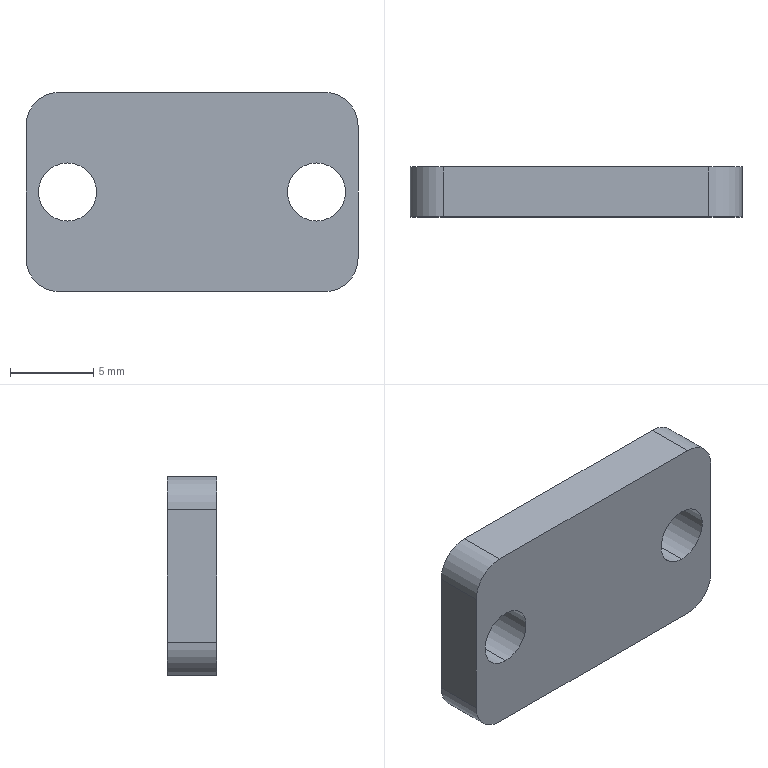Part | STEP file | MGN9C short slider pad plate 1001 | 1 solid | 14 faces | box 20 x 3 x 12 mm | volume 651.972 mm3 | cylinder 8 | plane 6 | commonest cylinder face diameters 3.5 x4 4 x4
STEP:
#1=CARTESIAN_POINT('',(0.,0.,0.));
#2=DIRECTION('',(0.,0.,1.));
#3=DIRECTION('',(1.,0.,0.));
#4=AXIS2_PLACEMENT_3D('',#1,#2,#3);
#5=CARTESIAN_POINT('',(7.5,3.,-1.75));
#6=VERTEX_POINT('',#5);
#7=CARTESIAN_POINT('',(7.5,0.,-1.75));
#8=VERTEX_POINT('',#7);
#9=CARTESIAN_POINT('',(7.5,3.,-1.75));
#10=DIRECTION('',(0.,-1.,0.));
#11=VECTOR('',#10,1.);
#12=LINE('',#9,#11);
#13=CARTESIAN_POINT('',(7.5,3.,0.));
#14=DIRECTION('',(0.,-1.,0.));
#15=DIRECTION('',(0.,0.,-1.));
#16=AXIS2_PLACEMENT_3D('',#13,#14,#15);
#17=CYLINDRICAL_SURFACE('',#16,1.75);
#18=CARTESIAN_POINT('',(6.283,0.));
#19=DIRECTION('',(0.,1.));
#20=VECTOR('',#19,1.);
#21=LINE('',#18,#20);
#22=(GEOMETRIC_REPRESENTATION_CONTEXT(2)PARAMETRIC_REPRESENTATION_CONTEXT()REPRESENTATION_CONTEXT('',''));
#23=DEFINITIONAL_REPRESENTATION('',(#21),#22);
#24=PCURVE('',#17,#23);
#25=CARTESIAN_POINT('',(7.5,3.,0.));
#26=DIRECTION('',(0.,-1.,0.));
#27=DIRECTION('',(0.,0.,-1.));
#28=AXIS2_PLACEMENT_3D('',#25,#26,#27);
#29=CYLINDRICAL_SURFACE('',#28,1.75);
#30=CARTESIAN_POINT('',(0.,0.));
#31=DIRECTION('',(0.,1.));
#32=VECTOR('',#31,1.);
#33=LINE('',#30,#32);
#34=(GEOMETRIC_REPRESENTATION_CONTEXT(2)PARAMETRIC_REPRESENTATION_CONTEXT()REPRESENTATION_CONTEXT('',''));
#35=DEFINITIONAL_REPRESENTATION('',(#33),#34);
#36=PCURVE('',#29,#35);
#37=SURFACE_CURVE('',#12,(#24,#36),.PCURVE_S1.);
#38=EDGE_CURVE('',#6,#8,#37,.T.);
#39=ORIENTED_EDGE('',*,*,#38,.T.);
#40=CARTESIAN_POINT('',(7.5,0.,1.75));
#41=VERTEX_POINT('',#40);
#42=CARTESIAN_POINT('',(7.5,0.,0.));
#43=DIRECTION('',(0.,1.,0.));
#44=DIRECTION('',(0.,0.,-1.));
#45=AXIS2_PLACEMENT_3D('',#42,#43,#44);
#46=CIRCLE('',#45,1.75);
#47=CARTESIAN_POINT('',(6.283,3.));
#48=DIRECTION('',(-1.,0.));
#49=VECTOR('',#48,1.);
#50=LINE('',#47,#49);
#51=(GEOMETRIC_REPRESENTATION_CONTEXT(2)PARAMETRIC_REPRESENTATION_CONTEXT()REPRESENTATION_CONTEXT('',''));
#52=DEFINITIONAL_REPRESENTATION('',(#50),#51);
#53=PCURVE('',#17,#52);
#54=CARTESIAN_POINT('',(0.,0.,0.));
#55=DIRECTION('',(0.,-1.,0.));
#56=DIRECTION('',(0.,0.,-1.));
#57=AXIS2_PLACEMENT_3D('',#54,#55,#56);
#58=PLANE('',#57);
#59=CARTESIAN_POINT('',(1.75,7.5));
#60=CARTESIAN_POINT('',(1.75,4.469));
#61=CARTESIAN_POINT('',(-0.875,5.984));
#62=CARTESIAN_POINT('',(-3.5,7.5));
#63=CARTESIAN_POINT('',(-0.875,9.016));
#64=CARTESIAN_POINT('',(1.75,10.531));
#65=CARTESIAN_POINT('',(1.75,7.5));
#66=(BOUNDED_CURVE()B_SPLINE_CURVE(2,(#59,#60,#61,#62,#63,#64,#65),.UNSPECIFIED.,.T.,.F.)B_SPLINE_CURVE_WITH_KNOTS((1,2,2,2,2,1),(-2.094,0.,2.094,4.189,6.283,8.378),.UNSPECIFIED.)CURVE()GEOMETRIC_REPRESENTATION_ITEM()RATIONAL_B_SPLINE_CURVE((1.,0.5,1.,0.5,1.,0.5,1.))REPRESENTATION_ITEM(''));
#67=(GEOMETRIC_REPRESENTATION_CONTEXT(2)PARAMETRIC_REPRESENTATION_CONTEXT()REPRESENTATION_CONTEXT('',''));
#68=DEFINITIONAL_REPRESENTATION('',(#66),#67);
#69=PCURVE('',#58,#68);
#70=SURFACE_CURVE('',#46,(#53,#69),.PCURVE_S1.);
#71=EDGE_CURVE('',#8,#41,#70,.T.);
#72=ORIENTED_EDGE('',*,*,#71,.T.);
#73=CARTESIAN_POINT('',(7.5,3.,1.75));
#74=VERTEX_POINT('',#73);
#75=CARTESIAN_POINT('',(7.5,3.,1.75));
#76=DIRECTION('',(0.,-1.,0.));
#77=VECTOR('',#76,1.);
#78=LINE('',#75,#77);
#79=CARTESIAN_POINT('',(3.142,0.));
#80=DIRECTION('',(0.,1.));
#81=VECTOR('',#80,1.);
#82=LINE('',#79,#81);
#83=(GEOMETRIC_REPRESENTATION_CONTEXT(2)PARAMETRIC_REPRESENTATION_CONTEXT()REPRESENTATION_CONTEXT('',''));
#84=DEFINITIONAL_REPRESENTATION('',(#82),#83);
#85=PCURVE('',#17,#84);
#86=CARTESIAN_POINT('',(3.142,0.));
#87=DIRECTION('',(0.,1.));
#88=VECTOR('',#87,1.);
#89=LINE('',#86,#88);
#90=(GEOMETRIC_REPRESENTATION_CONTEXT(2)PARAMETRIC_REPRESENTATION_CONTEXT()REPRESENTATION_CONTEXT('',''));
#91=DEFINITIONAL_REPRESENTATION('',(#89),#90);
#92=PCURVE('',#29,#91);
#93=SURFACE_CURVE('',#78,(#85,#92),.PCURVE_S1.);
#94=EDGE_CURVE('',#74,#41,#93,.T.);
#95=ORIENTED_EDGE('',*,*,#94,.F.);
#96=CARTESIAN_POINT('',(7.5,3.,0.));
#97=DIRECTION('',(0.,1.,0.));
#98=DIRECTION('',(0.,0.,-1.));
#99=AXIS2_PLACEMENT_3D('',#96,#97,#98);
#100=CIRCLE('',#99,1.75);
#101=CARTESIAN_POINT('',(6.283,0.));
#102=DIRECTION('',(-1.,0.));
#103=VECTOR('',#102,1.);
#104=LINE('',#101,#103);
#105=(GEOMETRIC_REPRESENTATION_CONTEXT(2)PARAMETRIC_REPRESENTATION_CONTEXT()REPRESENTATION_CONTEXT('',''));
#106=DEFINITIONAL_REPRESENTATION('',(#104),#105);
#107=PCURVE('',#17,#106);
#108=CARTESIAN_POINT('',(0.,3.,0.));
#109=DIRECTION('',(0.,-1.,0.));
#110=DIRECTION('',(0.,0.,-1.));
#111=AXIS2_PLACEMENT_3D('',#108,#109,#110);
#112=PLANE('',#111);
#113=CARTESIAN_POINT('',(1.75,7.5));
#114=CARTESIAN_POINT('',(1.75,4.469));
#115=CARTESIAN_POINT('',(-0.875,5.984));
#116=CARTESIAN_POINT('',(-3.5,7.5));
#117=CARTESIAN_POINT('',(-0.875,9.016));
#118=CARTESIAN_POINT('',(1.75,10.531));
#119=CARTESIAN_POINT('',(1.75,7.5));
#120=(BOUNDED_CURVE()B_SPLINE_CURVE(2,(#113,#114,#115,#116,#117,#118,#119),.UNSPECIFIED.,.T.,.F.)B_SPLINE_CURVE_WITH_KNOTS((1,2,2,2,2,1),(-2.094,0.,2.094,4.189,6.283,8.378),.UNSPECIFIED.)CURVE()GEOMETRIC_REPRESENTATION_ITEM()RATIONAL_B_SPLINE_CURVE((1.,0.5,1.,0.5,1.,0.5,1.))REPRESENTATION_ITEM(''));
#121=(GEOMETRIC_REPRESENTATION_CONTEXT(2)PARAMETRIC_REPRESENTATION_CONTEXT()REPRESENTATION_CONTEXT('',''));
#122=DEFINITIONAL_REPRESENTATION('',(#120),#121);
#123=PCURVE('',#112,#122);
#124=SURFACE_CURVE('',#100,(#107,#123),.PCURVE_S1.);
#125=EDGE_CURVE('',#6,#74,#124,.T.);
#126=ORIENTED_EDGE('',*,*,#125,.F.);
#127=EDGE_LOOP('',(#39,#72,#95,#126));
#128=FACE_BOUND('',#127,.F.);
#129=ADVANCED_FACE('',(#128),#17,.F.);
#130=CARTESIAN_POINT('',(-7.5,3.,-1.75));
#131=VERTEX_POINT('',#130);
#132=CARTESIAN_POINT('',(-7.5,0.,-1.75));
#133=VERTEX_POINT('',#132);
#134=CARTESIAN_POINT('',(-7.5,3.,-1.75));
#135=DIRECTION('',(0.,-1.,0.));
#136=VECTOR('',#135,1.);
#137=LINE('',#134,#136);
#138=CARTESIAN_POINT('',(-7.5,3.,0.));
#139=DIRECTION('',(0.,-1.,0.));
#140=DIRECTION('',(0.,0.,-1.));
#141=AXIS2_PLACEMENT_3D('',#138,#139,#140);
#142=CYLINDRICAL_SURFACE('',#141,1.75);
#143=CARTESIAN_POINT('',(6.283,0.));
#144=DIRECTION('',(0.,1.));
#145=VECTOR('',#144,1.);
#146=LINE('',#143,#145);
#147=(GEOMETRIC_REPRESENTATION_CONTEXT(2)PARAMETRIC_REPRESENTATION_CONTEXT()REPRESENTATION_CONTEXT('',''));
#148=DEFINITIONAL_REPRESENTATION('',(#146),#147);
#149=PCURVE('',#142,#148);
#150=CARTESIAN_POINT('',(-7.5,3.,0.));
#151=DIRECTION('',(0.,-1.,0.));
#152=DIRECTION('',(0.,0.,-1.));
#153=AXIS2_PLACEMENT_3D('',#150,#151,#152);
#154=CYLINDRICAL_SURFACE('',#153,1.75);
#155=CARTESIAN_POINT('',(0.,0.));
#156=DIRECTION('',(0.,1.));
#157=VECTOR('',#156,1.);
#158=LINE('',#155,#157);
#159=(GEOMETRIC_REPRESENTATION_CONTEXT(2)PARAMETRIC_REPRESENTATION_CONTEXT()REPRESENTATION_CONTEXT('',''));
#160=DEFINITIONAL_REPRESENTATION('',(#158),#159);
#161=PCURVE('',#154,#160);
#162=SURFACE_CURVE('',#137,(#149,#161),.PCURVE_S1.);
#163=EDGE_CURVE('',#131,#133,#162,.T.);
#164=ORIENTED_EDGE('',*,*,#163,.T.);
#165=CARTESIAN_POINT('',(-7.5,0.,1.75));
#166=VERTEX_POINT('',#165);
#167=CARTESIAN_POINT('',(-7.5,0.,0.));
#168=DIRECTION('',(0.,1.,0.));
#169=DIRECTION('',(0.,0.,1.));
#170=AXIS2_PLACEMENT_3D('',#167,#168,#169);
#171=CIRCLE('',#170,1.75);
#172=CARTESIAN_POINT('',(9.425,3.));
#173=DIRECTION('',(-1.,0.));
#174=VECTOR('',#173,1.);
#175=LINE('',#172,#174);
#176=(GEOMETRIC_REPRESENTATION_CONTEXT(2)PARAMETRIC_REPRESENTATION_CONTEXT()REPRESENTATION_CONTEXT('',''));
#177=DEFINITIONAL_REPRESENTATION('',(#175),#176);
#178=PCURVE('',#142,#177);
#179=CARTESIAN_POINT('',(-1.75,-7.5));
#180=CARTESIAN_POINT('',(-1.75,-4.469));
#181=CARTESIAN_POINT('',(0.875,-5.984));
#182=CARTESIAN_POINT('',(3.5,-7.5));
#183=CARTESIAN_POINT('',(0.875,-9.016));
#184=CARTESIAN_POINT('',(-1.75,-10.531));
#185=CARTESIAN_POINT('',(-1.75,-7.5));
#186=(BOUNDED_CURVE()B_SPLINE_CURVE(2,(#179,#180,#181,#182,#183,#184,#185),.UNSPECIFIED.,.T.,.F.)B_SPLINE_CURVE_WITH_KNOTS((1,2,2,2,2,1),(-2.094,0.,2.094,4.189,6.283,8.378),.UNSPECIFIED.)CURVE()GEOMETRIC_REPRESENTATION_ITEM()RATIONAL_B_SPLINE_CURVE((1.,0.5,1.,0.5,1.,0.5,1.))REPRESENTATION_ITEM(''));
#187=(GEOMETRIC_REPRESENTATION_CONTEXT(2)PARAMETRIC_REPRESENTATION_CONTEXT()REPRESENTATION_CONTEXT('',''));
#188=DEFINITIONAL_REPRESENTATION('',(#186),#187);
#189=PCURVE('',#58,#188);
#190=SURFACE_CURVE('',#171,(#178,#189),.PCURVE_S1.);
#191=EDGE_CURVE('',#133,#166,#190,.T.);
#192=ORIENTED_EDGE('',*,*,#191,.T.);
#193=CARTESIAN_POINT('',(-7.5,3.,1.75));
#194=VERTEX_POINT('',#193);
#195=CARTESIAN_POINT('',(-7.5,3.,1.75));
#196=DIRECTION('',(0.,-1.,0.));
#197=VECTOR('',#196,1.);
#198=LINE('',#195,#197);
#199=CARTESIAN_POINT('',(3.142,0.));
#200=DIRECTION('',(0.,1.));
#201=VECTOR('',#200,1.);
#202=LINE('',#199,#201);
#203=(GEOMETRIC_REPRESENTATION_CONTEXT(2)PARAMETRIC_REPRESENTATION_CONTEXT()REPRESENTATION_CONTEXT('',''));
#204=DEFINITIONAL_REPRESENTATION('',(#202),#203);
#205=PCURVE('',#142,#204);
#206=CARTESIAN_POINT('',(3.142,0.));
#207=DIRECTION('',(0.,1.));
#208=VECTOR('',#207,1.);
#209=LINE('',#206,#208);
#210=(GEOMETRIC_REPRESENTATION_CONTEXT(2)PARAMETRIC_REPRESENTATION_CONTEXT()REPRESENTATION_CONTEXT('',''));
#211=DEFINITIONAL_REPRESENTATION('',(#209),#210);
#212=PCURVE('',#154,#211);
#213=SURFACE_CURVE('',#198,(#205,#212),.PCURVE_S1.);
#214=EDGE_CURVE('',#194,#166,#213,.T.);
#215=ORIENTED_EDGE('',*,*,#214,.F.);
#216=CARTESIAN_POINT('',(-7.5,3.,0.));
#217=DIRECTION('',(0.,1.,0.));
#218=DIRECTION('',(0.,0.,1.));
#219=AXIS2_PLACEMENT_3D('',#216,#217,#218);
#220=CIRCLE('',#219,1.75);
#221=CARTESIAN_POINT('',(9.425,0.));
#222=DIRECTION('',(-1.,0.));
#223=VECTOR('',#222,1.);
#224=LINE('',#221,#223);
#225=(GEOMETRIC_REPRESENTATION_CONTEXT(2)PARAMETRIC_REPRESENTATION_CONTEXT()REPRESENTATION_CONTEXT('',''));
#226=DEFINITIONAL_REPRESENTATION('',(#224),#225);
#227=PCURVE('',#142,#226);
#228=CARTESIAN_POINT('',(-1.75,-7.5));
#229=CARTESIAN_POINT('',(-1.75,-4.469));
#230=CARTESIAN_POINT('',(0.875,-5.984));
#231=CARTESIAN_POINT('',(3.5,-7.5));
#232=CARTESIAN_POINT('',(0.875,-9.016));
#233=CARTESIAN_POINT('',(-1.75,-10.531));
#234=CARTESIAN_POINT('',(-1.75,-7.5));
#235=(BOUNDED_CURVE()B_SPLINE_CURVE(2,(#228,#229,#230,#231,#232,#233,#234),.UNSPECIFIED.,.T.,.F.)B_SPLINE_CURVE_WITH_KNOTS((1,2,2,2,2,1),(-2.094,0.,2.094,4.189,6.283,8.378),.UNSPECIFIED.)CURVE()GEOMETRIC_REPRESENTATION_ITEM()RATIONAL_B_SPLINE_CURVE((1.,0.5,1.,0.5,1.,0.5,1.))REPRESENTATION_ITEM(''));
#236=(GEOMETRIC_REPRESENTATION_CONTEXT(2)PARAMETRIC_REPRESENTATION_CONTEXT()REPRESENTATION_CONTEXT('',''));
#237=DEFINITIONAL_REPRESENTATION('',(#235),#236);
#238=PCURVE('',#112,#237);
#239=SURFACE_CURVE('',#220,(#227,#238),.PCURVE_S1.);
#240=EDGE_CURVE('',#131,#194,#239,.T.);
#241=ORIENTED_EDGE('',*,*,#240,.F.);
#242=EDGE_LOOP('',(#164,#192,#215,#241));
#243=FACE_BOUND('',#242,.F.);
#244=ADVANCED_FACE('',(#243),#142,.F.);
#245=CARTESIAN_POINT('',(-10.,3.,-4.));
#246=VERTEX_POINT('',#245);
#247=CARTESIAN_POINT('',(-10.,3.,4.));
#248=VERTEX_POINT('',#247);
#249=CARTESIAN_POINT('',(-10.,3.,6.));
#250=DIRECTION('',(0.,0.,1.));
#251=VECTOR('',#250,1.);
#252=LINE('',#249,#251);
#253=CARTESIAN_POINT('',(-6.,-10.));
#254=DIRECTION('',(-1.,0.));
#255=VECTOR('',#254,1.);
#256=LINE('',#253,#255);
#257=(GEOMETRIC_REPRESENTATION_CONTEXT(2)PARAMETRIC_REPRESENTATION_CONTEXT()REPRESENTATION_CONTEXT('',''));
#258=DEFINITIONAL_REPRESENTATION('',(#256),#257);
#259=PCURVE('',#112,#258);
#260=CARTESIAN_POINT('',(-10.,3.,6.));
#261=DIRECTION('',(1.,0.,0.));
#262=DIRECTION('',(0.,0.,-1.));
#263=AXIS2_PLACEMENT_3D('',#260,#261,#262);
#264=PLANE('',#263);
#265=CARTESIAN_POINT('',(0.,0.));
#266=DIRECTION('',(-1.,0.));
#267=VECTOR('',#266,1.);
#268=LINE('',#265,#267);
#269=(GEOMETRIC_REPRESENTATION_CONTEXT(2)PARAMETRIC_REPRESENTATION_CONTEXT()REPRESENTATION_CONTEXT('',''));
#270=DEFINITIONAL_REPRESENTATION('',(#268),#269);
#271=PCURVE('',#264,#270);
#272=SURFACE_CURVE('',#252,(#259,#271),.PCURVE_S1.);
#273=EDGE_CURVE('',#246,#248,#272,.T.);
#274=ORIENTED_EDGE('',*,*,#273,.T.);
#275=CARTESIAN_POINT('',(-8.,3.,6.));
#276=VERTEX_POINT('',#275);
#277=CARTESIAN_POINT('',(-8.,3.,4.));
#278=DIRECTION('',(0.,1.,0.));
#279=DIRECTION('',(0.,0.,-1.));
#280=AXIS2_PLACEMENT_3D('',#277,#278,#279);
#281=CIRCLE('',#280,2.);
#282=CARTESIAN_POINT('',(-2.,-8.));
#283=CARTESIAN_POINT('',(-2.,-11.464));
#284=CARTESIAN_POINT('',(-5.,-9.732));
#285=CARTESIAN_POINT('',(-8.,-8.));
#286=CARTESIAN_POINT('',(-5.,-6.268));
#287=CARTESIAN_POINT('',(-2.,-4.536));
#288=CARTESIAN_POINT('',(-2.,-8.));
#289=(BOUNDED_CURVE()B_SPLINE_CURVE(2,(#282,#283,#284,#285,#286,#287,#288),.UNSPECIFIED.,.T.,.F.)B_SPLINE_CURVE_WITH_KNOTS((1,2,2,2,2,1),(-2.094,0.,2.094,4.189,6.283,8.378),.UNSPECIFIED.)CURVE()GEOMETRIC_REPRESENTATION_ITEM()RATIONAL_B_SPLINE_CURVE((1.,0.5,1.,0.5,1.,0.5,1.))REPRESENTATION_ITEM(''));
#290=(GEOMETRIC_REPRESENTATION_CONTEXT(2)PARAMETRIC_REPRESENTATION_CONTEXT()REPRESENTATION_CONTEXT('',''));
#291=DEFINITIONAL_REPRESENTATION('',(#289),#290);
#292=PCURVE('',#112,#291);
#293=CARTESIAN_POINT('',(-8.,3.,4.));
#294=DIRECTION('',(0.,-1.,0.));
#295=DIRECTION('',(0.,0.,-1.));
#296=AXIS2_PLACEMENT_3D('',#293,#294,#295);
#297=CYLINDRICAL_SURFACE('',#296,2.);
#298=CARTESIAN_POINT('',(6.283,0.));
#299=DIRECTION('',(-1.,0.));
#300=VECTOR('',#299,1.);
#301=LINE('',#298,#300);
#302=(GEOMETRIC_REPRESENTATION_CONTEXT(2)PARAMETRIC_REPRESENTATION_CONTEXT()REPRESENTATION_CONTEXT('',''));
#303=DEFINITIONAL_REPRESENTATION('',(#301),#302);
#304=PCURVE('',#297,#303);
#305=SURFACE_CURVE('',#281,(#292,#304),.PCURVE_S1.);
#306=EDGE_CURVE('',#248,#276,#305,.T.);
#307=ORIENTED_EDGE('',*,*,#306,.T.);
#308=CARTESIAN_POINT('',(8.,3.,6.));
#309=VERTEX_POINT('',#308);
#310=CARTESIAN_POINT('',(-10.,3.,6.));
#311=DIRECTION('',(1.,0.,0.));
#312=VECTOR('',#311,1.);
#313=LINE('',#310,#312);
#314=CARTESIAN_POINT('',(-6.,-10.));
#315=DIRECTION('',(0.,1.));
#316=VECTOR('',#315,1.);
#317=LINE('',#314,#316);
#318=(GEOMETRIC_REPRESENTATION_CONTEXT(2)PARAMETRIC_REPRESENTATION_CONTEXT()REPRESENTATION_CONTEXT('',''));
#319=DEFINITIONAL_REPRESENTATION('',(#317),#318);
#320=PCURVE('',#112,#319);
#321=CARTESIAN_POINT('',(-10.,3.,6.));
#322=DIRECTION('',(0.,0.,-1.));
#323=DIRECTION('',(-1.,0.,0.));
#324=AXIS2_PLACEMENT_3D('',#321,#322,#323);
#325=PLANE('',#324);
#326=CARTESIAN_POINT('',(0.,0.));
#327=DIRECTION('',(-1.,0.));
#328=VECTOR('',#327,1.);
#329=LINE('',#326,#328);
#330=(GEOMETRIC_REPRESENTATION_CONTEXT(2)PARAMETRIC_REPRESENTATION_CONTEXT()REPRESENTATION_CONTEXT('',''));
#331=DEFINITIONAL_REPRESENTATION('',(#329),#330);
#332=PCURVE('',#325,#331);
#333=SURFACE_CURVE('',#313,(#320,#332),.PCURVE_S1.);
#334=EDGE_CURVE('',#276,#309,#333,.T.);
#335=ORIENTED_EDGE('',*,*,#334,.T.);
#336=CARTESIAN_POINT('',(10.,3.,4.));
#337=VERTEX_POINT('',#336);
#338=CARTESIAN_POINT('',(8.,3.,4.));
#339=DIRECTION('',(0.,1.,0.));
#340=DIRECTION('',(0.,0.,-1.));
#341=AXIS2_PLACEMENT_3D('',#338,#339,#340);
#342=CIRCLE('',#341,2.);
#343=CARTESIAN_POINT('',(-2.,8.));
#344=CARTESIAN_POINT('',(-2.,4.536));
#345=CARTESIAN_POINT('',(-5.,6.268));
#346=CARTESIAN_POINT('',(-8.,8.));
#347=CARTESIAN_POINT('',(-5.,9.732));
#348=CARTESIAN_POINT('',(-2.,11.464));
#349=CARTESIAN_POINT('',(-2.,8.));
#350=(BOUNDED_CURVE()B_SPLINE_CURVE(2,(#343,#344,#345,#346,#347,#348,#349),.UNSPECIFIED.,.T.,.F.)B_SPLINE_CURVE_WITH_KNOTS((1,2,2,2,2,1),(-2.094,0.,2.094,4.189,6.283,8.378),.UNSPECIFIED.)CURVE()GEOMETRIC_REPRESENTATION_ITEM()RATIONAL_B_SPLINE_CURVE((1.,0.5,1.,0.5,1.,0.5,1.))REPRESENTATION_ITEM(''));
#351=(GEOMETRIC_REPRESENTATION_CONTEXT(2)PARAMETRIC_REPRESENTATION_CONTEXT()REPRESENTATION_CONTEXT('',''));
#352=DEFINITIONAL_REPRESENTATION('',(#350),#351);
#353=PCURVE('',#112,#352);
#354=CARTESIAN_POINT('',(8.,3.,4.));
#355=DIRECTION('',(0.,-1.,0.));
#356=DIRECTION('',(0.,0.,-1.));
#357=AXIS2_PLACEMENT_3D('',#354,#355,#356);
#358=CYLINDRICAL_SURFACE('',#357,2.);
#359=CARTESIAN_POINT('',(6.283,0.));
#360=DIRECTION('',(-1.,0.));
#361=VECTOR('',#360,1.);
#362=LINE('',#359,#361);
#363=(GEOMETRIC_REPRESENTATION_CONTEXT(2)PARAMETRIC_REPRESENTATION_CONTEXT()REPRESENTATION_CONTEXT('',''));
#364=DEFINITIONAL_REPRESENTATION('',(#362),#363);
#365=PCURVE('',#358,#364);
#366=SURFACE_CURVE('',#342,(#353,#365),.PCURVE_S1.);
#367=EDGE_CURVE('',#309,#337,#366,.T.);
#368=ORIENTED_EDGE('',*,*,#367,.T.);
#369=CARTESIAN_POINT('',(10.,3.,-4.));
#370=VERTEX_POINT('',#369);
#371=CARTESIAN_POINT('',(10.,3.,6.));
#372=DIRECTION('',(0.,0.,-1.));
#373=VECTOR('',#372,1.);
#374=LINE('',#371,#373);
#375=CARTESIAN_POINT('',(-6.,10.));
#376=DIRECTION('',(1.,0.));
#377=VECTOR('',#376,1.);
#378=LINE('',#375,#377);
#379=(GEOMETRIC_REPRESENTATION_CONTEXT(2)PARAMETRIC_REPRESENTATION_CONTEXT()REPRESENTATION_CONTEXT('',''));
#380=DEFINITIONAL_REPRESENTATION('',(#378),#379);
#381=PCURVE('',#112,#380);
#382=CARTESIAN_POINT('',(10.,3.,6.));
#383=DIRECTION('',(-1.,0.,0.));
#384=DIRECTION('',(0.,0.,1.));
#385=AXIS2_PLACEMENT_3D('',#382,#383,#384);
#386=PLANE('',#385);
#387=CARTESIAN_POINT('',(0.,0.));
#388=DIRECTION('',(-1.,0.));
#389=VECTOR('',#388,1.);
#390=LINE('',#387,#389);
#391=(GEOMETRIC_REPRESENTATION_CONTEXT(2)PARAMETRIC_REPRESENTATION_CONTEXT()REPRESENTATION_CONTEXT('',''));
#392=DEFINITIONAL_REPRESENTATION('',(#390),#391);
#393=PCURVE('',#386,#392);
#394=SURFACE_CURVE('',#374,(#381,#393),.PCURVE_S1.);
#395=EDGE_CURVE('',#337,#370,#394,.T.);
#396=ORIENTED_EDGE('',*,*,#395,.T.);
#397=CARTESIAN_POINT('',(8.,3.,-6.));
#398=VERTEX_POINT('',#397);
#399=CARTESIAN_POINT('',(8.,3.,-4.));
#400=DIRECTION('',(0.,1.,0.));
#401=DIRECTION('',(0.,0.,-1.));
#402=AXIS2_PLACEMENT_3D('',#399,#400,#401);
#403=CIRCLE('',#402,2.);
#404=CARTESIAN_POINT('',(6.,8.));
#405=CARTESIAN_POINT('',(6.,4.536));
#406=CARTESIAN_POINT('',(3.,6.268));
#407=CARTESIAN_POINT('',(0.,8.));
#408=CARTESIAN_POINT('',(3.,9.732));
#409=CARTESIAN_POINT('',(6.,11.464));
#410=CARTESIAN_POINT('',(6.,8.));
#411=(BOUNDED_CURVE()B_SPLINE_CURVE(2,(#404,#405,#406,#407,#408,#409,#410),.UNSPECIFIED.,.T.,.F.)B_SPLINE_CURVE_WITH_KNOTS((1,2,2,2,2,1),(-2.094,0.,2.094,4.189,6.283,8.378),.UNSPECIFIED.)CURVE()GEOMETRIC_REPRESENTATION_ITEM()RATIONAL_B_SPLINE_CURVE((1.,0.5,1.,0.5,1.,0.5,1.))REPRESENTATION_ITEM(''));
#412=(GEOMETRIC_REPRESENTATION_CONTEXT(2)PARAMETRIC_REPRESENTATION_CONTEXT()REPRESENTATION_CONTEXT('',''));
#413=DEFINITIONAL_REPRESENTATION('',(#411),#412);
#414=PCURVE('',#112,#413);
#415=CARTESIAN_POINT('',(8.,3.,-4.));
#416=DIRECTION('',(0.,-1.,0.));
#417=DIRECTION('',(0.,0.,-1.));
#418=AXIS2_PLACEMENT_3D('',#415,#416,#417);
#419=CYLINDRICAL_SURFACE('',#418,2.);
#420=CARTESIAN_POINT('',(6.283,0.));
#421=DIRECTION('',(-1.,0.));
#422=VECTOR('',#421,1.);
#423=LINE('',#420,#422);
#424=(GEOMETRIC_REPRESENTATION_CONTEXT(2)PARAMETRIC_REPRESENTATION_CONTEXT()REPRESENTATION_CONTEXT('',''));
#425=DEFINITIONAL_REPRESENTATION('',(#423),#424);
#426=PCURVE('',#419,#425);
#427=SURFACE_CURVE('',#403,(#414,#426),.PCURVE_S1.);
#428=EDGE_CURVE('',#370,#398,#427,.T.);
#429=ORIENTED_EDGE('',*,*,#428,.T.);
#430=CARTESIAN_POINT('',(-8.,3.,-6.));
#431=VERTEX_POINT('',#430);
#432=CARTESIAN_POINT('',(-10.,3.,-6.));
#433=DIRECTION('',(-1.,0.,0.));
#434=VECTOR('',#433,1.);
#435=LINE('',#432,#434);
#436=CARTESIAN_POINT('',(6.,-10.));
#437=DIRECTION('',(0.,-1.));
#438=VECTOR('',#437,1.);
#439=LINE('',#436,#438);
#440=(GEOMETRIC_REPRESENTATION_CONTEXT(2)PARAMETRIC_REPRESENTATION_CONTEXT()REPRESENTATION_CONTEXT('',''));
#441=DEFINITIONAL_REPRESENTATION('',(#439),#440);
#442=PCURVE('',#112,#441);
#443=CARTESIAN_POINT('',(-10.,3.,-6.));
#444=DIRECTION('',(0.,0.,1.));
#445=DIRECTION('',(1.,0.,0.));
#446=AXIS2_PLACEMENT_3D('',#443,#444,#445);
#447=PLANE('',#446);
#448=CARTESIAN_POINT('',(0.,0.));
#449=DIRECTION('',(-1.,0.));
#450=VECTOR('',#449,1.);
#451=LINE('',#448,#450);
#452=(GEOMETRIC_REPRESENTATION_CONTEXT(2)PARAMETRIC_REPRESENTATION_CONTEXT()REPRESENTATION_CONTEXT('',''));
#453=DEFINITIONAL_REPRESENTATION('',(#451),#452);
#454=PCURVE('',#447,#453);
#455=SURFACE_CURVE('',#435,(#442,#454),.PCURVE_S1.);
#456=EDGE_CURVE('',#398,#431,#455,.T.);
#457=ORIENTED_EDGE('',*,*,#456,.T.);
#458=CARTESIAN_POINT('',(-8.,3.,-4.));
#459=DIRECTION('',(0.,1.,0.));
#460=DIRECTION('',(0.,0.,-1.));
#461=AXIS2_PLACEMENT_3D('',#458,#459,#460);
#462=CIRCLE('',#461,2.);
#463=CARTESIAN_POINT('',(6.,-8.));
#464=CARTESIAN_POINT('',(6.,-11.464));
#465=CARTESIAN_POINT('',(3.,-9.732));
#466=CARTESIAN_POINT('',(0.,-8.));
#467=CARTESIAN_POINT('',(3.,-6.268));
#468=CARTESIAN_POINT('',(6.,-4.536));
#469=CARTESIAN_POINT('',(6.,-8.));
#470=(BOUNDED_CURVE()B_SPLINE_CURVE(2,(#463,#464,#465,#466,#467,#468,#469),.UNSPECIFIED.,.T.,.F.)B_SPLINE_CURVE_WITH_KNOTS((1,2,2,2,2,1),(-2.094,0.,2.094,4.189,6.283,8.378),.UNSPECIFIED.)CURVE()GEOMETRIC_REPRESENTATION_ITEM()RATIONAL_B_SPLINE_CURVE((1.,0.5,1.,0.5,1.,0.5,1.))REPRESENTATION_ITEM(''));
#471=(GEOMETRIC_REPRESENTATION_CONTEXT(2)PARAMETRIC_REPRESENTATION_CONTEXT()REPRESENTATION_CONTEXT('',''));
#472=DEFINITIONAL_REPRESENTATION('',(#470),#471);
#473=PCURVE('',#112,#472);
#474=CARTESIAN_POINT('',(-8.,3.,-4.));
#475=DIRECTION('',(0.,-1.,0.));
#476=DIRECTION('',(0.,0.,-1.));
#477=AXIS2_PLACEMENT_3D('',#474,#475,#476);
#478=CYLINDRICAL_SURFACE('',#477,2.);
#479=CARTESIAN_POINT('',(6.283,0.));
#480=DIRECTION('',(-1.,0.));
#481=VECTOR('',#480,1.);
#482=LINE('',#479,#481);
#483=(GEOMETRIC_REPRESENTATION_CONTEXT(2)PARAMETRIC_REPRESENTATION_CONTEXT()REPRESENTATION_CONTEXT('',''));
#484=DEFINITIONAL_REPRESENTATION('',(#482),#483);
#485=PCURVE('',#478,#484);
#486=SURFACE_CURVE('',#462,(#473,#485),.PCURVE_S1.);
#487=EDGE_CURVE('',#431,#246,#486,.T.);
#488=ORIENTED_EDGE('',*,*,#487,.T.);
#489=EDGE_LOOP('',(#274,#307,#335,#368,#396,#429,#457,#488));
#490=FACE_BOUND('',#489,.T.);
#491=ORIENTED_EDGE('',*,*,#240,.F.);
#492=CARTESIAN_POINT('',(-7.5,3.,0.));
#493=DIRECTION('',(0.,1.,0.));
#494=DIRECTION('',(0.,0.,1.));
#495=AXIS2_PLACEMENT_3D('',#492,#493,#494);
#496=CIRCLE('',#495,1.75);
#497=CARTESIAN_POINT('',(-1.75,-7.5));
#498=CARTESIAN_POINT('',(-1.75,-4.469));
#499=CARTESIAN_POINT('',(0.875,-5.984));
#500=CARTESIAN_POINT('',(3.5,-7.5));
#501=CARTESIAN_POINT('',(0.875,-9.016));
#502=CARTESIAN_POINT('',(-1.75,-10.531));
#503=CARTESIAN_POINT('',(-1.75,-7.5));
#504=(BOUNDED_CURVE()B_SPLINE_CURVE(2,(#497,#498,#499,#500,#501,#502,#503),.UNSPECIFIED.,.T.,.F.)B_SPLINE_CURVE_WITH_KNOTS((1,2,2,2,2,1),(-2.094,0.,2.094,4.189,6.283,8.378),.UNSPECIFIED.)CURVE()GEOMETRIC_REPRESENTATION_ITEM()RATIONAL_B_SPLINE_CURVE((1.,0.5,1.,0.5,1.,0.5,1.))REPRESENTATION_ITEM(''));
#505=(GEOMETRIC_REPRESENTATION_CONTEXT(2)PARAMETRIC_REPRESENTATION_CONTEXT()REPRESENTATION_CONTEXT('',''));
#506=DEFINITIONAL_REPRESENTATION('',(#504),#505);
#507=PCURVE('',#112,#506);
#508=CARTESIAN_POINT('',(3.142,0.));
#509=DIRECTION('',(-1.,0.));
#510=VECTOR('',#509,1.);
#511=LINE('',#508,#510);
#512=(GEOMETRIC_REPRESENTATION_CONTEXT(2)PARAMETRIC_REPRESENTATION_CONTEXT()REPRESENTATION_CONTEXT('',''));
#513=DEFINITIONAL_REPRESENTATION('',(#511),#512);
#514=PCURVE('',#154,#513);
#515=SURFACE_CURVE('',#496,(#507,#514),.PCURVE_S1.);
#516=EDGE_CURVE('',#194,#131,#515,.T.);
#517=ORIENTED_EDGE('',*,*,#516,.F.);
#518=EDGE_LOOP('',(#491,#517));
#519=FACE_BOUND('',#518,.T.);
#520=ORIENTED_EDGE('',*,*,#125,.F.);
#521=CARTESIAN_POINT('',(7.5,3.,0.));
#522=DIRECTION('',(0.,1.,0.));
#523=DIRECTION('',(0.,0.,-1.));
#524=AXIS2_PLACEMENT_3D('',#521,#522,#523);
#525=CIRCLE('',#524,1.75);
#526=CARTESIAN_POINT('',(1.75,7.5));
#527=CARTESIAN_POINT('',(1.75,4.469));
#528=CARTESIAN_POINT('',(-0.875,5.984));
#529=CARTESIAN_POINT('',(-3.5,7.5));
#530=CARTESIAN_POINT('',(-0.875,9.016));
#531=CARTESIAN_POINT('',(1.75,10.531));
#532=CARTESIAN_POINT('',(1.75,7.5));
#533=(BOUNDED_CURVE()B_SPLINE_CURVE(2,(#526,#527,#528,#529,#530,#531,#532),.UNSPECIFIED.,.T.,.F.)B_SPLINE_CURVE_WITH_KNOTS((1,2,2,2,2,1),(-2.094,0.,2.094,4.189,6.283,8.378),.UNSPECIFIED.)CURVE()GEOMETRIC_REPRESENTATION_ITEM()RATIONAL_B_SPLINE_CURVE((1.,0.5,1.,0.5,1.,0.5,1.))REPRESENTATION_ITEM(''));
#534=(GEOMETRIC_REPRESENTATION_CONTEXT(2)PARAMETRIC_REPRESENTATION_CONTEXT()REPRESENTATION_CONTEXT('',''));
#535=DEFINITIONAL_REPRESENTATION('',(#533),#534);
#536=PCURVE('',#112,#535);
#537=CARTESIAN_POINT('',(6.283,0.));
#538=DIRECTION('',(-1.,0.));
#539=VECTOR('',#538,1.);
#540=LINE('',#537,#539);
#541=(GEOMETRIC_REPRESENTATION_CONTEXT(2)PARAMETRIC_REPRESENTATION_CONTEXT()REPRESENTATION_CONTEXT('',''));
#542=DEFINITIONAL_REPRESENTATION('',(#540),#541);
#543=PCURVE('',#29,#542);
#544=SURFACE_CURVE('',#525,(#536,#543),.PCURVE_S1.);
#545=EDGE_CURVE('',#74,#6,#544,.T.);
#546=ORIENTED_EDGE('',*,*,#545,.F.);
#547=EDGE_LOOP('',(#520,#546));
#548=FACE_BOUND('',#547,.T.);
#549=ADVANCED_FACE('',(#490,#519,#548),#112,.F.);
#550=ORIENTED_EDGE('',*,*,#191,.T.);
#551=CARTESIAN_POINT('',(-7.5,0.,0.));
#552=DIRECTION('',(0.,1.,0.));
#553=DIRECTION('',(0.,0.,1.));
#554=AXIS2_PLACEMENT_3D('',#551,#552,#553);
#555=CIRCLE('',#554,1.75);
#556=CARTESIAN_POINT('',(-1.75,-7.5));
#557=CARTESIAN_POINT('',(-1.75,-4.469));
#558=CARTESIAN_POINT('',(0.875,-5.984));
#559=CARTESIAN_POINT('',(3.5,-7.5));
#560=CARTESIAN_POINT('',(0.875,-9.016));
#561=CARTESIAN_POINT('',(-1.75,-10.531));
#562=CARTESIAN_POINT('',(-1.75,-7.5));
#563=(BOUNDED_CURVE()B_SPLINE_CURVE(2,(#556,#557,#558,#559,#560,#561,#562),.UNSPECIFIED.,.T.,.F.)B_SPLINE_CURVE_WITH_KNOTS((1,2,2,2,2,1),(-2.094,0.,2.094,4.189,6.283,8.378),.UNSPECIFIED.)CURVE()GEOMETRIC_REPRESENTATION_ITEM()RATIONAL_B_SPLINE_CURVE((1.,0.5,1.,0.5,1.,0.5,1.))REPRESENTATION_ITEM(''));
#564=(GEOMETRIC_REPRESENTATION_CONTEXT(2)PARAMETRIC_REPRESENTATION_CONTEXT()REPRESENTATION_CONTEXT('',''));
#565=DEFINITIONAL_REPRESENTATION('',(#563),#564);
#566=PCURVE('',#58,#565);
#567=CARTESIAN_POINT('',(3.142,3.));
#568=DIRECTION('',(-1.,0.));
#569=VECTOR('',#568,1.);
#570=LINE('',#567,#569);
#571=(GEOMETRIC_REPRESENTATION_CONTEXT(2)PARAMETRIC_REPRESENTATION_CONTEXT()REPRESENTATION_CONTEXT('',''));
#572=DEFINITIONAL_REPRESENTATION('',(#570),#571);
#573=PCURVE('',#154,#572);
#574=SURFACE_CURVE('',#555,(#566,#573),.PCURVE_S1.);
#575=EDGE_CURVE('',#166,#133,#574,.T.);
#576=ORIENTED_EDGE('',*,*,#575,.T.);
#577=EDGE_LOOP('',(#550,#576));
#578=FACE_BOUND('',#577,.T.);
#579=CARTESIAN_POINT('',(-8.,0.,6.));
#580=VERTEX_POINT('',#579);
#581=CARTESIAN_POINT('',(8.,0.,6.));
#582=VERTEX_POINT('',#581);
#583=CARTESIAN_POINT('',(-10.,0.,6.));
#584=DIRECTION('',(1.,0.,0.));
#585=VECTOR('',#584,1.);
#586=LINE('',#583,#585);
#587=CARTESIAN_POINT('',(-6.,-10.));
#588=DIRECTION('',(0.,1.));
#589=VECTOR('',#588,1.);
#590=LINE('',#587,#589);
#591=(GEOMETRIC_REPRESENTATION_CONTEXT(2)PARAMETRIC_REPRESENTATION_CONTEXT()REPRESENTATION_CONTEXT('',''));
#592=DEFINITIONAL_REPRESENTATION('',(#590),#591);
#593=PCURVE('',#58,#592);
#594=CARTESIAN_POINT('',(0.,-3.));
#595=DIRECTION('',(-1.,0.));
#596=VECTOR('',#595,1.);
#597=LINE('',#594,#596);
#598=(GEOMETRIC_REPRESENTATION_CONTEXT(2)PARAMETRIC_REPRESENTATION_CONTEXT()REPRESENTATION_CONTEXT('',''));
#599=DEFINITIONAL_REPRESENTATION('',(#597),#598);
#600=PCURVE('',#325,#599);
#601=SURFACE_CURVE('',#586,(#593,#600),.PCURVE_S1.);
#602=EDGE_CURVE('',#580,#582,#601,.T.);
#603=ORIENTED_EDGE('',*,*,#602,.F.);
#604=CARTESIAN_POINT('',(-10.,0.,4.));
#605=VERTEX_POINT('',#604);
#606=CARTESIAN_POINT('',(-8.,0.,4.));
#607=DIRECTION('',(0.,-1.,0.));
#608=DIRECTION('',(0.,0.,-1.));
#609=AXIS2_PLACEMENT_3D('',#606,#607,#608);
#610=CIRCLE('',#609,2.);
#611=CARTESIAN_POINT('',(-4.,-8.));
#612=DIRECTION('',(1.,0.));
#613=AXIS2_PLACEMENT_2D('',#611,#612);
#614=CIRCLE('',#613,2.);
#615=(GEOMETRIC_REPRESENTATION_CONTEXT(2)PARAMETRIC_REPRESENTATION_CONTEXT()REPRESENTATION_CONTEXT('',''));
#616=DEFINITIONAL_REPRESENTATION('',(#614),#615);
#617=PCURVE('',#58,#616);
#618=CARTESIAN_POINT('',(0.,3.));
#619=DIRECTION('',(1.,0.));
#620=VECTOR('',#619,1.);
#621=LINE('',#618,#620);
#622=(GEOMETRIC_REPRESENTATION_CONTEXT(2)PARAMETRIC_REPRESENTATION_CONTEXT()REPRESENTATION_CONTEXT('',''));
#623=DEFINITIONAL_REPRESENTATION('',(#621),#622);
#624=PCURVE('',#297,#623);
#625=SURFACE_CURVE('',#610,(#617,#624),.PCURVE_S1.);
#626=EDGE_CURVE('',#580,#605,#625,.T.);
#627=ORIENTED_EDGE('',*,*,#626,.T.);
#628=CARTESIAN_POINT('',(-10.,0.,-4.));
#629=VERTEX_POINT('',#628);
#630=CARTESIAN_POINT('',(-10.,0.,6.));
#631=DIRECTION('',(0.,0.,1.));
#632=VECTOR('',#631,1.);
#633=LINE('',#630,#632);
#634=CARTESIAN_POINT('',(-6.,-10.));
#635=DIRECTION('',(-1.,0.));
#636=VECTOR('',#635,1.);
#637=LINE('',#634,#636);
#638=(GEOMETRIC_REPRESENTATION_CONTEXT(2)PARAMETRIC_REPRESENTATION_CONTEXT()REPRESENTATION_CONTEXT('',''));
#639=DEFINITIONAL_REPRESENTATION('',(#637),#638);
#640=PCURVE('',#58,#639);
#641=CARTESIAN_POINT('',(0.,-3.));
#642=DIRECTION('',(-1.,0.));
#643=VECTOR('',#642,1.);
#644=LINE('',#641,#643);
#645=(GEOMETRIC_REPRESENTATION_CONTEXT(2)PARAMETRIC_REPRESENTATION_CONTEXT()REPRESENTATION_CONTEXT('',''));
#646=DEFINITIONAL_REPRESENTATION('',(#644),#645);
#647=PCURVE('',#264,#646);
#648=SURFACE_CURVE('',#633,(#640,#647),.PCURVE_S1.);
#649=EDGE_CURVE('',#629,#605,#648,.T.);
#650=ORIENTED_EDGE('',*,*,#649,.F.);
#651=CARTESIAN_POINT('',(-8.,0.,-6.));
#652=VERTEX_POINT('',#651);
#653=CARTESIAN_POINT('',(-8.,0.,-4.));
#654=DIRECTION('',(0.,-1.,0.));
#655=DIRECTION('',(0.,0.,-1.));
#656=AXIS2_PLACEMENT_3D('',#653,#654,#655);
#657=CIRCLE('',#656,2.);
#658=CARTESIAN_POINT('',(4.,-8.));
#659=DIRECTION('',(1.,0.));
#660=AXIS2_PLACEMENT_2D('',#658,#659);
#661=CIRCLE('',#660,2.);
#662=(GEOMETRIC_REPRESENTATION_CONTEXT(2)PARAMETRIC_REPRESENTATION_CONTEXT()REPRESENTATION_CONTEXT('',''));
#663=DEFINITIONAL_REPRESENTATION('',(#661),#662);
#664=PCURVE('',#58,#663);
#665=CARTESIAN_POINT('',(0.,3.));
#666=DIRECTION('',(1.,0.));
#667=VECTOR('',#666,1.);
#668=LINE('',#665,#667);
#669=(GEOMETRIC_REPRESENTATION_CONTEXT(2)PARAMETRIC_REPRESENTATION_CONTEXT()REPRESENTATION_CONTEXT('',''));
#670=DEFINITIONAL_REPRESENTATION('',(#668),#669);
#671=PCURVE('',#478,#670);
#672=SURFACE_CURVE('',#657,(#664,#671),.PCURVE_S1.);
#673=EDGE_CURVE('',#629,#652,#672,.T.);
#674=ORIENTED_EDGE('',*,*,#673,.T.);
#675=CARTESIAN_POINT('',(8.,0.,-6.));
#676=VERTEX_POINT('',#675);
#677=CARTESIAN_POINT('',(-10.,0.,-6.));
#678=DIRECTION('',(-1.,0.,0.));
#679=VECTOR('',#678,1.);
#680=LINE('',#677,#679);
#681=CARTESIAN_POINT('',(6.,-10.));
#682=DIRECTION('',(0.,-1.));
#683=VECTOR('',#682,1.);
#684=LINE('',#681,#683);
#685=(GEOMETRIC_REPRESENTATION_CONTEXT(2)PARAMETRIC_REPRESENTATION_CONTEXT()REPRESENTATION_CONTEXT('',''));
#686=DEFINITIONAL_REPRESENTATION('',(#684),#685);
#687=PCURVE('',#58,#686);
#688=CARTESIAN_POINT('',(0.,-3.));
#689=DIRECTION('',(-1.,0.));
#690=VECTOR('',#689,1.);
#691=LINE('',#688,#690);
#692=(GEOMETRIC_REPRESENTATION_CONTEXT(2)PARAMETRIC_REPRESENTATION_CONTEXT()REPRESENTATION_CONTEXT('',''));
#693=DEFINITIONAL_REPRESENTATION('',(#691),#692);
#694=PCURVE('',#447,#693);
#695=SURFACE_CURVE('',#680,(#687,#694),.PCURVE_S1.);
#696=EDGE_CURVE('',#676,#652,#695,.T.);
#697=ORIENTED_EDGE('',*,*,#696,.F.);
#698=CARTESIAN_POINT('',(10.,0.,-4.));
#699=VERTEX_POINT('',#698);
#700=CARTESIAN_POINT('',(8.,0.,-4.));
#701=DIRECTION('',(0.,-1.,0.));
#702=DIRECTION('',(0.,0.,-1.));
#703=AXIS2_PLACEMENT_3D('',#700,#701,#702);
#704=CIRCLE('',#703,2.);
#705=CARTESIAN_POINT('',(4.,8.));
#706=DIRECTION('',(1.,0.));
#707=AXIS2_PLACEMENT_2D('',#705,#706);
#708=CIRCLE('',#707,2.);
#709=(GEOMETRIC_REPRESENTATION_CONTEXT(2)PARAMETRIC_REPRESENTATION_CONTEXT()REPRESENTATION_CONTEXT('',''));
#710=DEFINITIONAL_REPRESENTATION('',(#708),#709);
#711=PCURVE('',#58,#710);
#712=CARTESIAN_POINT('',(0.,3.));
#713=DIRECTION('',(1.,0.));
#714=VECTOR('',#713,1.);
#715=LINE('',#712,#714);
#716=(GEOMETRIC_REPRESENTATION_CONTEXT(2)PARAMETRIC_REPRESENTATION_CONTEXT()REPRESENTATION_CONTEXT('',''));
#717=DEFINITIONAL_REPRESENTATION('',(#715),#716);
#718=PCURVE('',#419,#717);
#719=SURFACE_CURVE('',#704,(#711,#718),.PCURVE_S1.);
#720=EDGE_CURVE('',#676,#699,#719,.T.);
#721=ORIENTED_EDGE('',*,*,#720,.T.);
#722=CARTESIAN_POINT('',(10.,0.,4.));
#723=VERTEX_POINT('',#722);
#724=CARTESIAN_POINT('',(10.,0.,6.));
#725=DIRECTION('',(0.,0.,-1.));
#726=VECTOR('',#725,1.);
#727=LINE('',#724,#726);
#728=CARTESIAN_POINT('',(-6.,10.));
#729=DIRECTION('',(1.,0.));
#730=VECTOR('',#729,1.);
#731=LINE('',#728,#730);
#732=(GEOMETRIC_REPRESENTATION_CONTEXT(2)PARAMETRIC_REPRESENTATION_CONTEXT()REPRESENTATION_CONTEXT('',''));
#733=DEFINITIONAL_REPRESENTATION('',(#731),#732);
#734=PCURVE('',#58,#733);
#735=CARTESIAN_POINT('',(0.,-3.));
#736=DIRECTION('',(-1.,0.));
#737=VECTOR('',#736,1.);
#738=LINE('',#735,#737);
#739=(GEOMETRIC_REPRESENTATION_CONTEXT(2)PARAMETRIC_REPRESENTATION_CONTEXT()REPRESENTATION_CONTEXT('',''));
#740=DEFINITIONAL_REPRESENTATION('',(#738),#739);
#741=PCURVE('',#386,#740);
#742=SURFACE_CURVE('',#727,(#734,#741),.PCURVE_S1.);
#743=EDGE_CURVE('',#723,#699,#742,.T.);
#744=ORIENTED_EDGE('',*,*,#743,.F.);
#745=CARTESIAN_POINT('',(8.,0.,4.));
#746=DIRECTION('',(0.,-1.,0.));
#747=DIRECTION('',(0.,0.,-1.));
#748=AXIS2_PLACEMENT_3D('',#745,#746,#747);
#749=CIRCLE('',#748,2.);
#750=CARTESIAN_POINT('',(-4.,8.));
#751=DIRECTION('',(1.,0.));
#752=AXIS2_PLACEMENT_2D('',#750,#751);
#753=CIRCLE('',#752,2.);
#754=(GEOMETRIC_REPRESENTATION_CONTEXT(2)PARAMETRIC_REPRESENTATION_CONTEXT()REPRESENTATION_CONTEXT('',''));
#755=DEFINITIONAL_REPRESENTATION('',(#753),#754);
#756=PCURVE('',#58,#755);
#757=CARTESIAN_POINT('',(0.,3.));
#758=DIRECTION('',(1.,0.));
#759=VECTOR('',#758,1.);
#760=LINE('',#757,#759);
#761=(GEOMETRIC_REPRESENTATION_CONTEXT(2)PARAMETRIC_REPRESENTATION_CONTEXT()REPRESENTATION_CONTEXT('',''));
#762=DEFINITIONAL_REPRESENTATION('',(#760),#761);
#763=PCURVE('',#358,#762);
#764=SURFACE_CURVE('',#749,(#756,#763),.PCURVE_S1.);
#765=EDGE_CURVE('',#723,#582,#764,.T.);
#766=ORIENTED_EDGE('',*,*,#765,.T.);
#767=EDGE_LOOP('',(#603,#627,#650,#674,#697,#721,#744,#766));
#768=FACE_BOUND('',#767,.T.);
#769=ORIENTED_EDGE('',*,*,#71,.T.);
#770=CARTESIAN_POINT('',(7.5,0.,0.));
#771=DIRECTION('',(0.,1.,0.));
#772=DIRECTION('',(0.,0.,-1.));
#773=AXIS2_PLACEMENT_3D('',#770,#771,#772);
#774=CIRCLE('',#773,1.75);
#775=CARTESIAN_POINT('',(1.75,7.5));
#776=CARTESIAN_POINT('',(1.75,4.469));
#777=CARTESIAN_POINT('',(-0.875,5.984));
#778=CARTESIAN_POINT('',(-3.5,7.5));
#779=CARTESIAN_POINT('',(-0.875,9.016));
#780=CARTESIAN_POINT('',(1.75,10.531));
#781=CARTESIAN_POINT('',(1.75,7.5));
#782=(BOUNDED_CURVE()B_SPLINE_CURVE(2,(#775,#776,#777,#778,#779,#780,#781),.UNSPECIFIED.,.T.,.F.)B_SPLINE_CURVE_WITH_KNOTS((1,2,2,2,2,1),(-2.094,0.,2.094,4.189,6.283,8.378),.UNSPECIFIED.)CURVE()GEOMETRIC_REPRESENTATION_ITEM()RATIONAL_B_SPLINE_CURVE((1.,0.5,1.,0.5,1.,0.5,1.))REPRESENTATION_ITEM(''));
#783=(GEOMETRIC_REPRESENTATION_CONTEXT(2)PARAMETRIC_REPRESENTATION_CONTEXT()REPRESENTATION_CONTEXT('',''));
#784=DEFINITIONAL_REPRESENTATION('',(#782),#783);
#785=PCURVE('',#58,#784);
#786=CARTESIAN_POINT('',(6.283,3.));
#787=DIRECTION('',(-1.,0.));
#788=VECTOR('',#787,1.);
#789=LINE('',#786,#788);
#790=(GEOMETRIC_REPRESENTATION_CONTEXT(2)PARAMETRIC_REPRESENTATION_CONTEXT()REPRESENTATION_CONTEXT('',''));
#791=DEFINITIONAL_REPRESENTATION('',(#789),#790);
#792=PCURVE('',#29,#791);
#793=SURFACE_CURVE('',#774,(#785,#792),.PCURVE_S1.);
#794=EDGE_CURVE('',#41,#8,#793,.T.);
#795=ORIENTED_EDGE('',*,*,#794,.T.);
#796=EDGE_LOOP('',(#769,#795));
#797=FACE_BOUND('',#796,.T.);
#798=ADVANCED_FACE('',(#578,#768,#797),#58,.T.);
#799=ORIENTED_EDGE('',*,*,#743,.T.);
#800=CARTESIAN_POINT('',(10.,3.,-4.));
#801=DIRECTION('',(0.,1.,0.));
#802=VECTOR('',#801,1.);
#803=LINE('',#800,#802);
#804=CARTESIAN_POINT('',(-10.,0.));
#805=DIRECTION('',(0.,1.));
#806=VECTOR('',#805,1.);
#807=LINE('',#804,#806);
#808=(GEOMETRIC_REPRESENTATION_CONTEXT(2)PARAMETRIC_REPRESENTATION_CONTEXT()REPRESENTATION_CONTEXT('',''));
#809=DEFINITIONAL_REPRESENTATION('',(#807),#808);
#810=PCURVE('',#386,#809);
#811=CARTESIAN_POINT('',(1.571,0.));
#812=DIRECTION('',(0.,-1.));
#813=VECTOR('',#812,1.);
#814=LINE('',#811,#813);
#815=(GEOMETRIC_REPRESENTATION_CONTEXT(2)PARAMETRIC_REPRESENTATION_CONTEXT()REPRESENTATION_CONTEXT('',''));
#816=DEFINITIONAL_REPRESENTATION('',(#814),#815);
#817=PCURVE('',#419,#816);
#818=SURFACE_CURVE('',#803,(#810,#817),.PCURVE_S1.);
#819=EDGE_CURVE('',#699,#370,#818,.T.);
#820=ORIENTED_EDGE('',*,*,#819,.T.);
#821=ORIENTED_EDGE('',*,*,#395,.F.);
#822=CARTESIAN_POINT('',(10.,3.,4.));
#823=DIRECTION('',(0.,-1.,0.));
#824=VECTOR('',#823,1.);
#825=LINE('',#822,#824);
#826=CARTESIAN_POINT('',(-2.,0.));
#827=DIRECTION('',(0.,-1.));
#828=VECTOR('',#827,1.);
#829=LINE('',#826,#828);
#830=(GEOMETRIC_REPRESENTATION_CONTEXT(2)PARAMETRIC_REPRESENTATION_CONTEXT()REPRESENTATION_CONTEXT('',''));
#831=DEFINITIONAL_REPRESENTATION('',(#829),#830);
#832=PCURVE('',#386,#831);
#833=CARTESIAN_POINT('',(1.571,0.));
#834=DIRECTION('',(0.,1.));
#835=VECTOR('',#834,1.);
#836=LINE('',#833,#835);
#837=(GEOMETRIC_REPRESENTATION_CONTEXT(2)PARAMETRIC_REPRESENTATION_CONTEXT()REPRESENTATION_CONTEXT('',''));
#838=DEFINITIONAL_REPRESENTATION('',(#836),#837);
#839=PCURVE('',#358,#838);
#840=SURFACE_CURVE('',#825,(#832,#839),.PCURVE_S1.);
#841=EDGE_CURVE('',#337,#723,#840,.T.);
#842=ORIENTED_EDGE('',*,*,#841,.T.);
#843=EDGE_LOOP('',(#799,#820,#821,#842));
#844=FACE_BOUND('',#843,.T.);
#845=ADVANCED_FACE('',(#844),#386,.F.);
#846=ORIENTED_EDGE('',*,*,#696,.T.);
#847=CARTESIAN_POINT('',(-8.,3.,-6.));
#848=DIRECTION('',(0.,1.,0.));
#849=VECTOR('',#848,1.);
#850=LINE('',#847,#849);
#851=CARTESIAN_POINT('',(2.,0.));
#852=DIRECTION('',(0.,1.));
#853=VECTOR('',#852,1.);
#854=LINE('',#851,#853);
#855=(GEOMETRIC_REPRESENTATION_CONTEXT(2)PARAMETRIC_REPRESENTATION_CONTEXT()REPRESENTATION_CONTEXT('',''));
#856=DEFINITIONAL_REPRESENTATION('',(#854),#855);
#857=PCURVE('',#447,#856);
#858=CARTESIAN_POINT('',(6.283,0.));
#859=DIRECTION('',(0.,-1.));
#860=VECTOR('',#859,1.);
#861=LINE('',#858,#860);
#862=(GEOMETRIC_REPRESENTATION_CONTEXT(2)PARAMETRIC_REPRESENTATION_CONTEXT()REPRESENTATION_CONTEXT('',''));
#863=DEFINITIONAL_REPRESENTATION('',(#861),#862);
#864=PCURVE('',#478,#863);
#865=SURFACE_CURVE('',#850,(#857,#864),.PCURVE_S1.);
#866=EDGE_CURVE('',#652,#431,#865,.T.);
#867=ORIENTED_EDGE('',*,*,#866,.T.);
#868=ORIENTED_EDGE('',*,*,#456,.F.);
#869=CARTESIAN_POINT('',(8.,3.,-6.));
#870=DIRECTION('',(0.,-1.,0.));
#871=VECTOR('',#870,1.);
#872=LINE('',#869,#871);
#873=CARTESIAN_POINT('',(18.,0.));
#874=DIRECTION('',(0.,-1.));
#875=VECTOR('',#874,1.);
#876=LINE('',#873,#875);
#877=(GEOMETRIC_REPRESENTATION_CONTEXT(2)PARAMETRIC_REPRESENTATION_CONTEXT()REPRESENTATION_CONTEXT('',''));
#878=DEFINITIONAL_REPRESENTATION('',(#876),#877);
#879=PCURVE('',#447,#878);
#880=CARTESIAN_POINT('',(0.,0.));
#881=DIRECTION('',(0.,1.));
#882=VECTOR('',#881,1.);
#883=LINE('',#880,#882);
#884=(GEOMETRIC_REPRESENTATION_CONTEXT(2)PARAMETRIC_REPRESENTATION_CONTEXT()REPRESENTATION_CONTEXT('',''));
#885=DEFINITIONAL_REPRESENTATION('',(#883),#884);
#886=PCURVE('',#419,#885);
#887=SURFACE_CURVE('',#872,(#879,#886),.PCURVE_S1.);
#888=EDGE_CURVE('',#398,#676,#887,.T.);
#889=ORIENTED_EDGE('',*,*,#888,.T.);
#890=EDGE_LOOP('',(#846,#867,#868,#889));
#891=FACE_BOUND('',#890,.T.);
#892=ADVANCED_FACE('',(#891),#447,.F.);
#893=ORIENTED_EDGE('',*,*,#649,.T.);
#894=CARTESIAN_POINT('',(-10.,3.,4.));
#895=DIRECTION('',(0.,1.,0.));
#896=VECTOR('',#895,1.);
#897=LINE('',#894,#896);
#898=CARTESIAN_POINT('',(2.,0.));
#899=DIRECTION('',(0.,1.));
#900=VECTOR('',#899,1.);
#901=LINE('',#898,#900);
#902=(GEOMETRIC_REPRESENTATION_CONTEXT(2)PARAMETRIC_REPRESENTATION_CONTEXT()REPRESENTATION_CONTEXT('',''));
#903=DEFINITIONAL_REPRESENTATION('',(#901),#902);
#904=PCURVE('',#264,#903);
#905=CARTESIAN_POINT('',(4.712,0.));
#906=DIRECTION('',(0.,-1.));
#907=VECTOR('',#906,1.);
#908=LINE('',#905,#907);
#909=(GEOMETRIC_REPRESENTATION_CONTEXT(2)PARAMETRIC_REPRESENTATION_CONTEXT()REPRESENTATION_CONTEXT('',''));
#910=DEFINITIONAL_REPRESENTATION('',(#908),#909);
#911=PCURVE('',#297,#910);
#912=SURFACE_CURVE('',#897,(#904,#911),.PCURVE_S1.);
#913=EDGE_CURVE('',#605,#248,#912,.T.);
#914=ORIENTED_EDGE('',*,*,#913,.T.);
#915=ORIENTED_EDGE('',*,*,#273,.F.);
#916=CARTESIAN_POINT('',(-10.,3.,-4.));
#917=DIRECTION('',(0.,-1.,0.));
#918=VECTOR('',#917,1.);
#919=LINE('',#916,#918);
#920=CARTESIAN_POINT('',(10.,0.));
#921=DIRECTION('',(0.,-1.));
#922=VECTOR('',#921,1.);
#923=LINE('',#920,#922);
#924=(GEOMETRIC_REPRESENTATION_CONTEXT(2)PARAMETRIC_REPRESENTATION_CONTEXT()REPRESENTATION_CONTEXT('',''));
#925=DEFINITIONAL_REPRESENTATION('',(#923),#924);
#926=PCURVE('',#264,#925);
#927=CARTESIAN_POINT('',(4.712,0.));
#928=DIRECTION('',(0.,1.));
#929=VECTOR('',#928,1.);
#930=LINE('',#927,#929);
#931=(GEOMETRIC_REPRESENTATION_CONTEXT(2)PARAMETRIC_REPRESENTATION_CONTEXT()REPRESENTATION_CONTEXT('',''));
#932=DEFINITIONAL_REPRESENTATION('',(#930),#931);
#933=PCURVE('',#478,#932);
#934=SURFACE_CURVE('',#919,(#926,#933),.PCURVE_S1.);
#935=EDGE_CURVE('',#246,#629,#934,.T.);
#936=ORIENTED_EDGE('',*,*,#935,.T.);
#937=EDGE_LOOP('',(#893,#914,#915,#936));
#938=FACE_BOUND('',#937,.T.);
#939=ADVANCED_FACE('',(#938),#264,.F.);
#940=ORIENTED_EDGE('',*,*,#334,.F.);
#941=CARTESIAN_POINT('',(-8.,3.,6.));
#942=DIRECTION('',(0.,-1.,0.));
#943=VECTOR('',#942,1.);
#944=LINE('',#941,#943);
#945=CARTESIAN_POINT('',(-2.,0.));
#946=DIRECTION('',(0.,-1.));
#947=VECTOR('',#946,1.);
#948=LINE('',#945,#947);
#949=(GEOMETRIC_REPRESENTATION_CONTEXT(2)PARAMETRIC_REPRESENTATION_CONTEXT()REPRESENTATION_CONTEXT('',''));
#950=DEFINITIONAL_REPRESENTATION('',(#948),#949);
#951=PCURVE('',#325,#950);
#952=CARTESIAN_POINT('',(3.142,0.));
#953=DIRECTION('',(0.,1.));
#954=VECTOR('',#953,1.);
#955=LINE('',#952,#954);
#956=(GEOMETRIC_REPRESENTATION_CONTEXT(2)PARAMETRIC_REPRESENTATION_CONTEXT()REPRESENTATION_CONTEXT('',''));
#957=DEFINITIONAL_REPRESENTATION('',(#955),#956);
#958=PCURVE('',#297,#957);
#959=SURFACE_CURVE('',#944,(#951,#958),.PCURVE_S1.);
#960=EDGE_CURVE('',#276,#580,#959,.T.);
#961=ORIENTED_EDGE('',*,*,#960,.T.);
#962=ORIENTED_EDGE('',*,*,#602,.T.);
#963=CARTESIAN_POINT('',(8.,3.,6.));
#964=DIRECTION('',(0.,1.,0.));
#965=VECTOR('',#964,1.);
#966=LINE('',#963,#965);
#967=CARTESIAN_POINT('',(-18.,0.));
#968=DIRECTION('',(0.,1.));
#969=VECTOR('',#968,1.);
#970=LINE('',#967,#969);
#971=(GEOMETRIC_REPRESENTATION_CONTEXT(2)PARAMETRIC_REPRESENTATION_CONTEXT()REPRESENTATION_CONTEXT('',''));
#972=DEFINITIONAL_REPRESENTATION('',(#970),#971);
#973=PCURVE('',#325,#972);
#974=CARTESIAN_POINT('',(3.142,0.));
#975=DIRECTION('',(0.,-1.));
#976=VECTOR('',#975,1.);
#977=LINE('',#974,#976);
#978=(GEOMETRIC_REPRESENTATION_CONTEXT(2)PARAMETRIC_REPRESENTATION_CONTEXT()REPRESENTATION_CONTEXT('',''));
#979=DEFINITIONAL_REPRESENTATION('',(#977),#978);
#980=PCURVE('',#358,#979);
#981=SURFACE_CURVE('',#966,(#973,#980),.PCURVE_S1.);
#982=EDGE_CURVE('',#582,#309,#981,.T.);
#983=ORIENTED_EDGE('',*,*,#982,.T.);
#984=EDGE_LOOP('',(#940,#961,#962,#983));
#985=FACE_BOUND('',#984,.T.);
#986=ADVANCED_FACE('',(#985),#325,.F.);
#987=ORIENTED_EDGE('',*,*,#575,.T.);
#988=ORIENTED_EDGE('',*,*,#163,.F.);
#989=ORIENTED_EDGE('',*,*,#516,.F.);
#990=ORIENTED_EDGE('',*,*,#214,.T.);
#991=EDGE_LOOP('',(#987,#988,#989,#990));
#992=FACE_BOUND('',#991,.F.);
#993=ADVANCED_FACE('',(#992),#154,.F.);
#994=ORIENTED_EDGE('',*,*,#794,.T.);
#995=ORIENTED_EDGE('',*,*,#38,.F.);
#996=ORIENTED_EDGE('',*,*,#545,.F.);
#997=ORIENTED_EDGE('',*,*,#94,.T.);
#998=EDGE_LOOP('',(#994,#995,#996,#997));
#999=FACE_BOUND('',#998,.F.);
#1000=ADVANCED_FACE('',(#999),#29,.F.);
#1001=ORIENTED_EDGE('',*,*,#306,.F.);
#1002=ORIENTED_EDGE('',*,*,#913,.F.);
#1003=ORIENTED_EDGE('',*,*,#626,.F.);
#1004=ORIENTED_EDGE('',*,*,#960,.F.);
#1005=EDGE_LOOP('',(#1001,#1002,#1003,#1004));
#1006=FACE_BOUND('',#1005,.T.);
#1007=ADVANCED_FACE('',(#1006),#297,.T.);
#1008=ORIENTED_EDGE('',*,*,#487,.F.);
#1009=ORIENTED_EDGE('',*,*,#866,.F.);
#1010=ORIENTED_EDGE('',*,*,#673,.F.);
#1011=ORIENTED_EDGE('',*,*,#935,.F.);
#1012=EDGE_LOOP('',(#1008,#1009,#1010,#1011));
#1013=FACE_BOUND('',#1012,.T.);
#1014=ADVANCED_FACE('',(#1013),#478,.T.);
#1015=ORIENTED_EDGE('',*,*,#428,.F.);
#1016=ORIENTED_EDGE('',*,*,#819,.F.);
#1017=ORIENTED_EDGE('',*,*,#720,.F.);
#1018=ORIENTED_EDGE('',*,*,#888,.F.);
#1019=EDGE_LOOP('',(#1015,#1016,#1017,#1018));
#1020=FACE_BOUND('',#1019,.T.);
#1021=ADVANCED_FACE('',(#1020),#419,.T.);
#1022=ORIENTED_EDGE('',*,*,#367,.F.);
#1023=ORIENTED_EDGE('',*,*,#982,.F.);
#1024=ORIENTED_EDGE('',*,*,#765,.F.);
#1025=ORIENTED_EDGE('',*,*,#841,.F.);
#1026=EDGE_LOOP('',(#1022,#1023,#1024,#1025));
#1027=FACE_BOUND('',#1026,.T.);
#1028=ADVANCED_FACE('',(#1027),#358,.T.);
#1029=CLOSED_SHELL('',(#129,#244,#549,#798,#845,#892,#939,#986,#993,#1000,#1007,#1014,#1021,#1028));
#1030=MANIFOLD_SOLID_BREP('',#1029);
#1031=(LENGTH_UNIT()NAMED_UNIT(*)SI_UNIT(.MILLI.,.METRE.));
#1032=UNCERTAINTY_MEASURE_WITH_UNIT(LENGTH_MEASURE(0.0000001),#1031,'','');
#1033=(NAMED_UNIT(*)PLANE_ANGLE_UNIT()SI_UNIT($,.RADIAN.));
#1034=(NAMED_UNIT(*)SI_UNIT($,.STERADIAN.)SOLID_ANGLE_UNIT());
#1035=(GEOMETRIC_REPRESENTATION_CONTEXT(3)GLOBAL_UNCERTAINTY_ASSIGNED_CONTEXT((#1032))GLOBAL_UNIT_ASSIGNED_CONTEXT((#1031,#1033,#1034))REPRESENTATION_CONTEXT('',''));
#1036=ADVANCED_BREP_SHAPE_REPRESENTATION('',(#4,#1030),#1035);